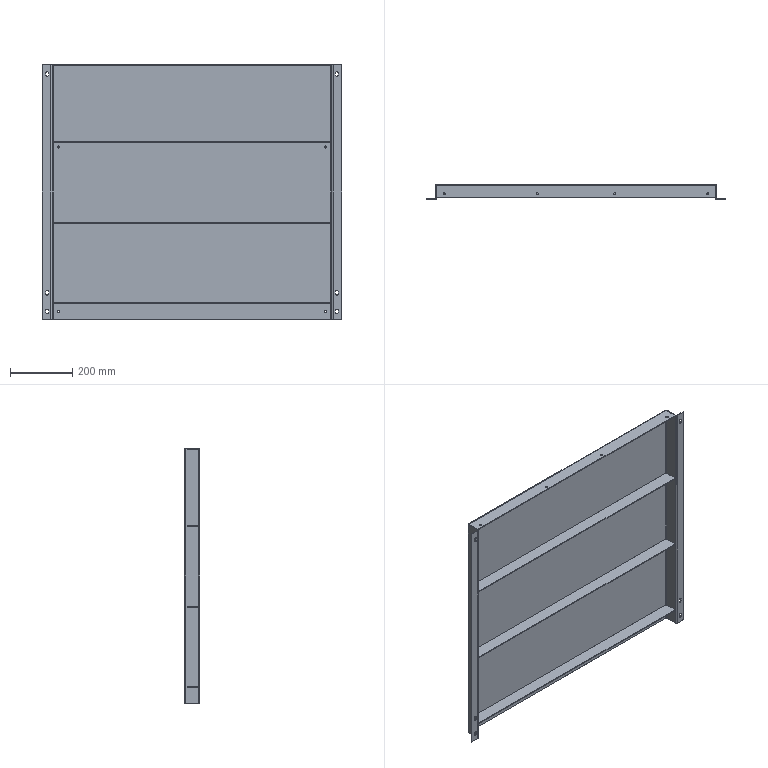Part | SolidWorks | features BaseBody 5, ICE 1 | 5 solids | 100 faces | box 966 x 49 x 820 mm | volume 3016837 mm3 | cylinder 50 | plane 50 | commonest cylinder face diameters 9 x18 7 x16 4 x12 10 x4